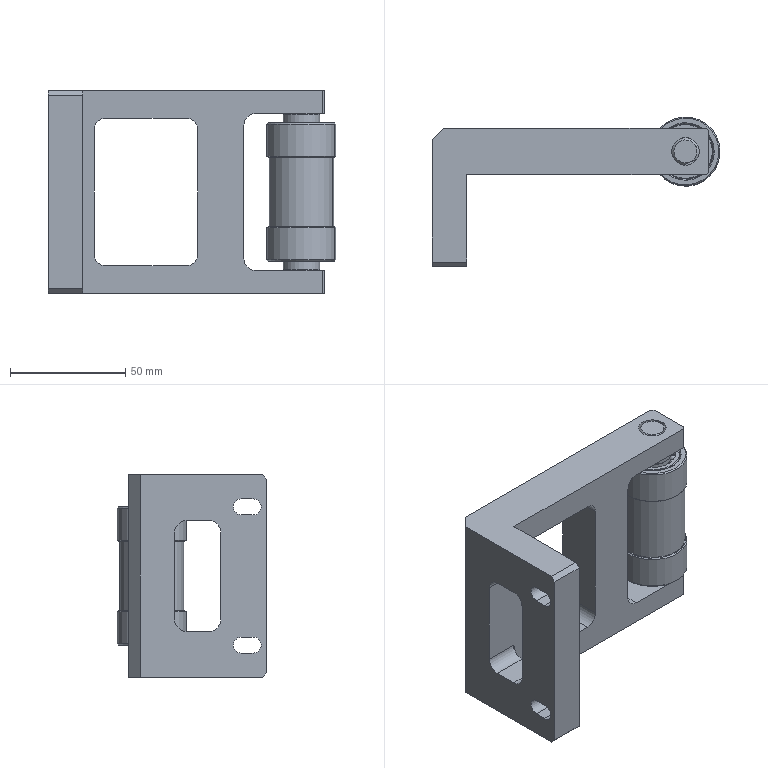Part | SolidWorks | features AEMSimFeature 1 | 7 solids | 348 faces | box 125 x 65 x 88 mm | volume 172222 mm3 | torus 124 | cylinder 68 | sphere 68 | plane 54 | cone 34 | commonest cylinder face diameters 16 x12 10 x10 12 x10 20 x10 24 x8 3.3 x4